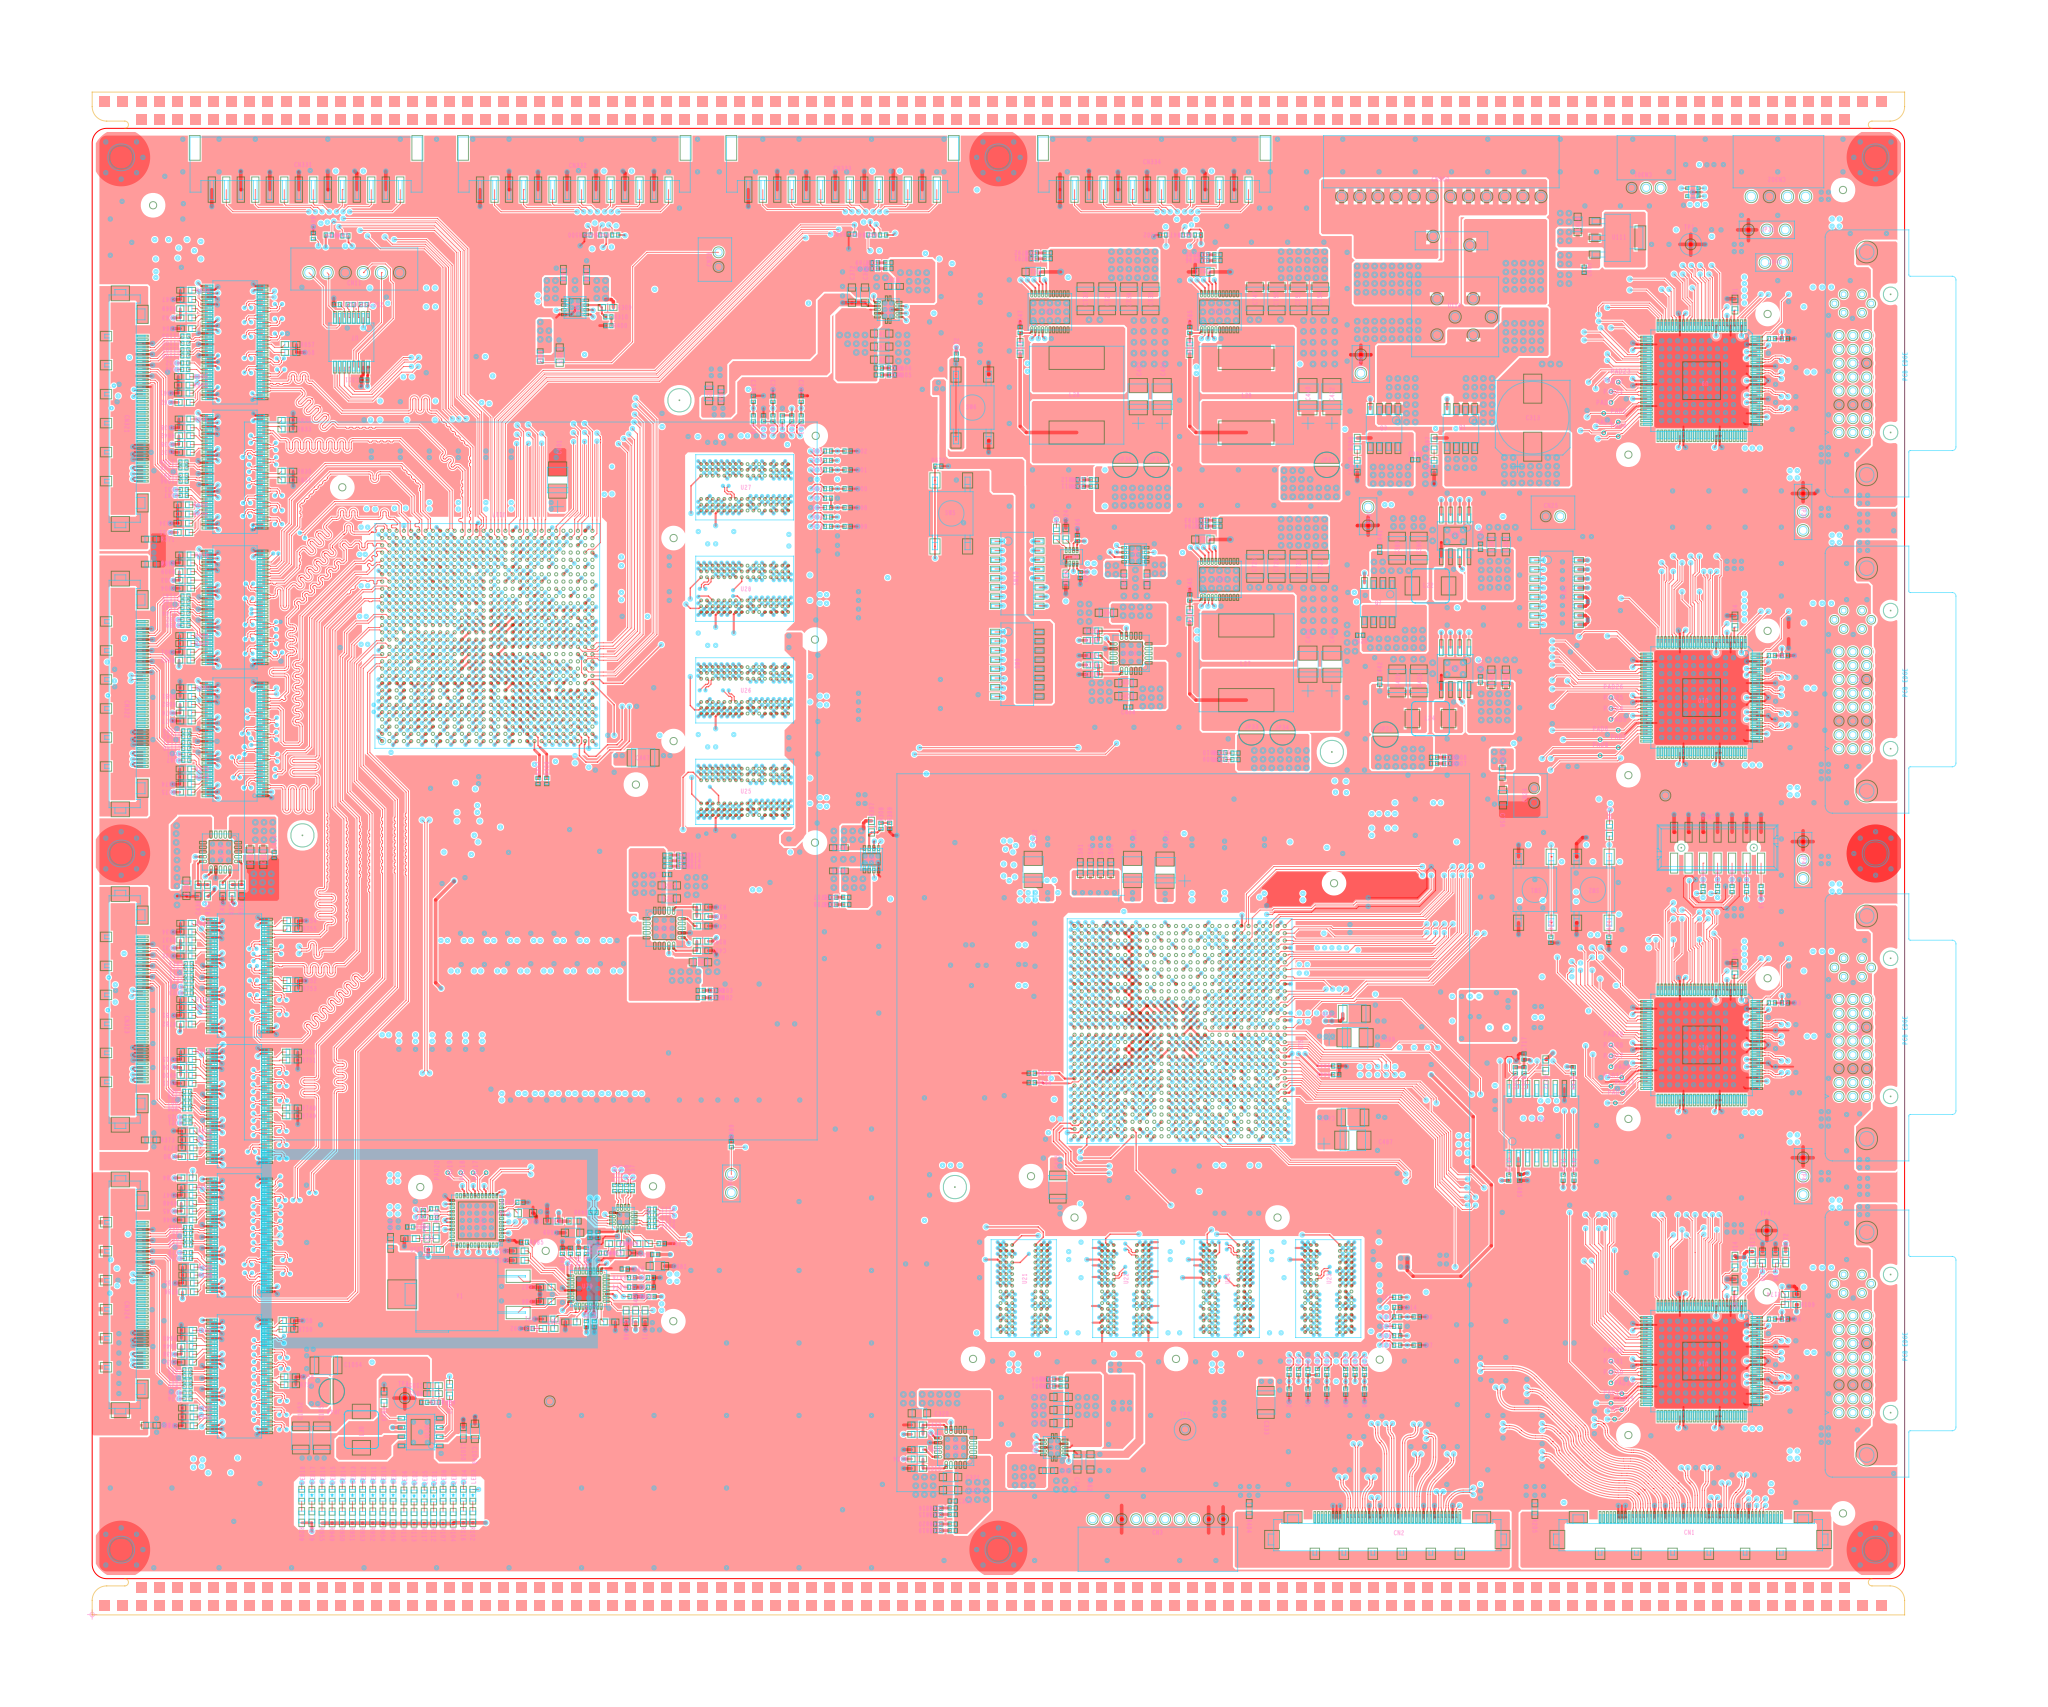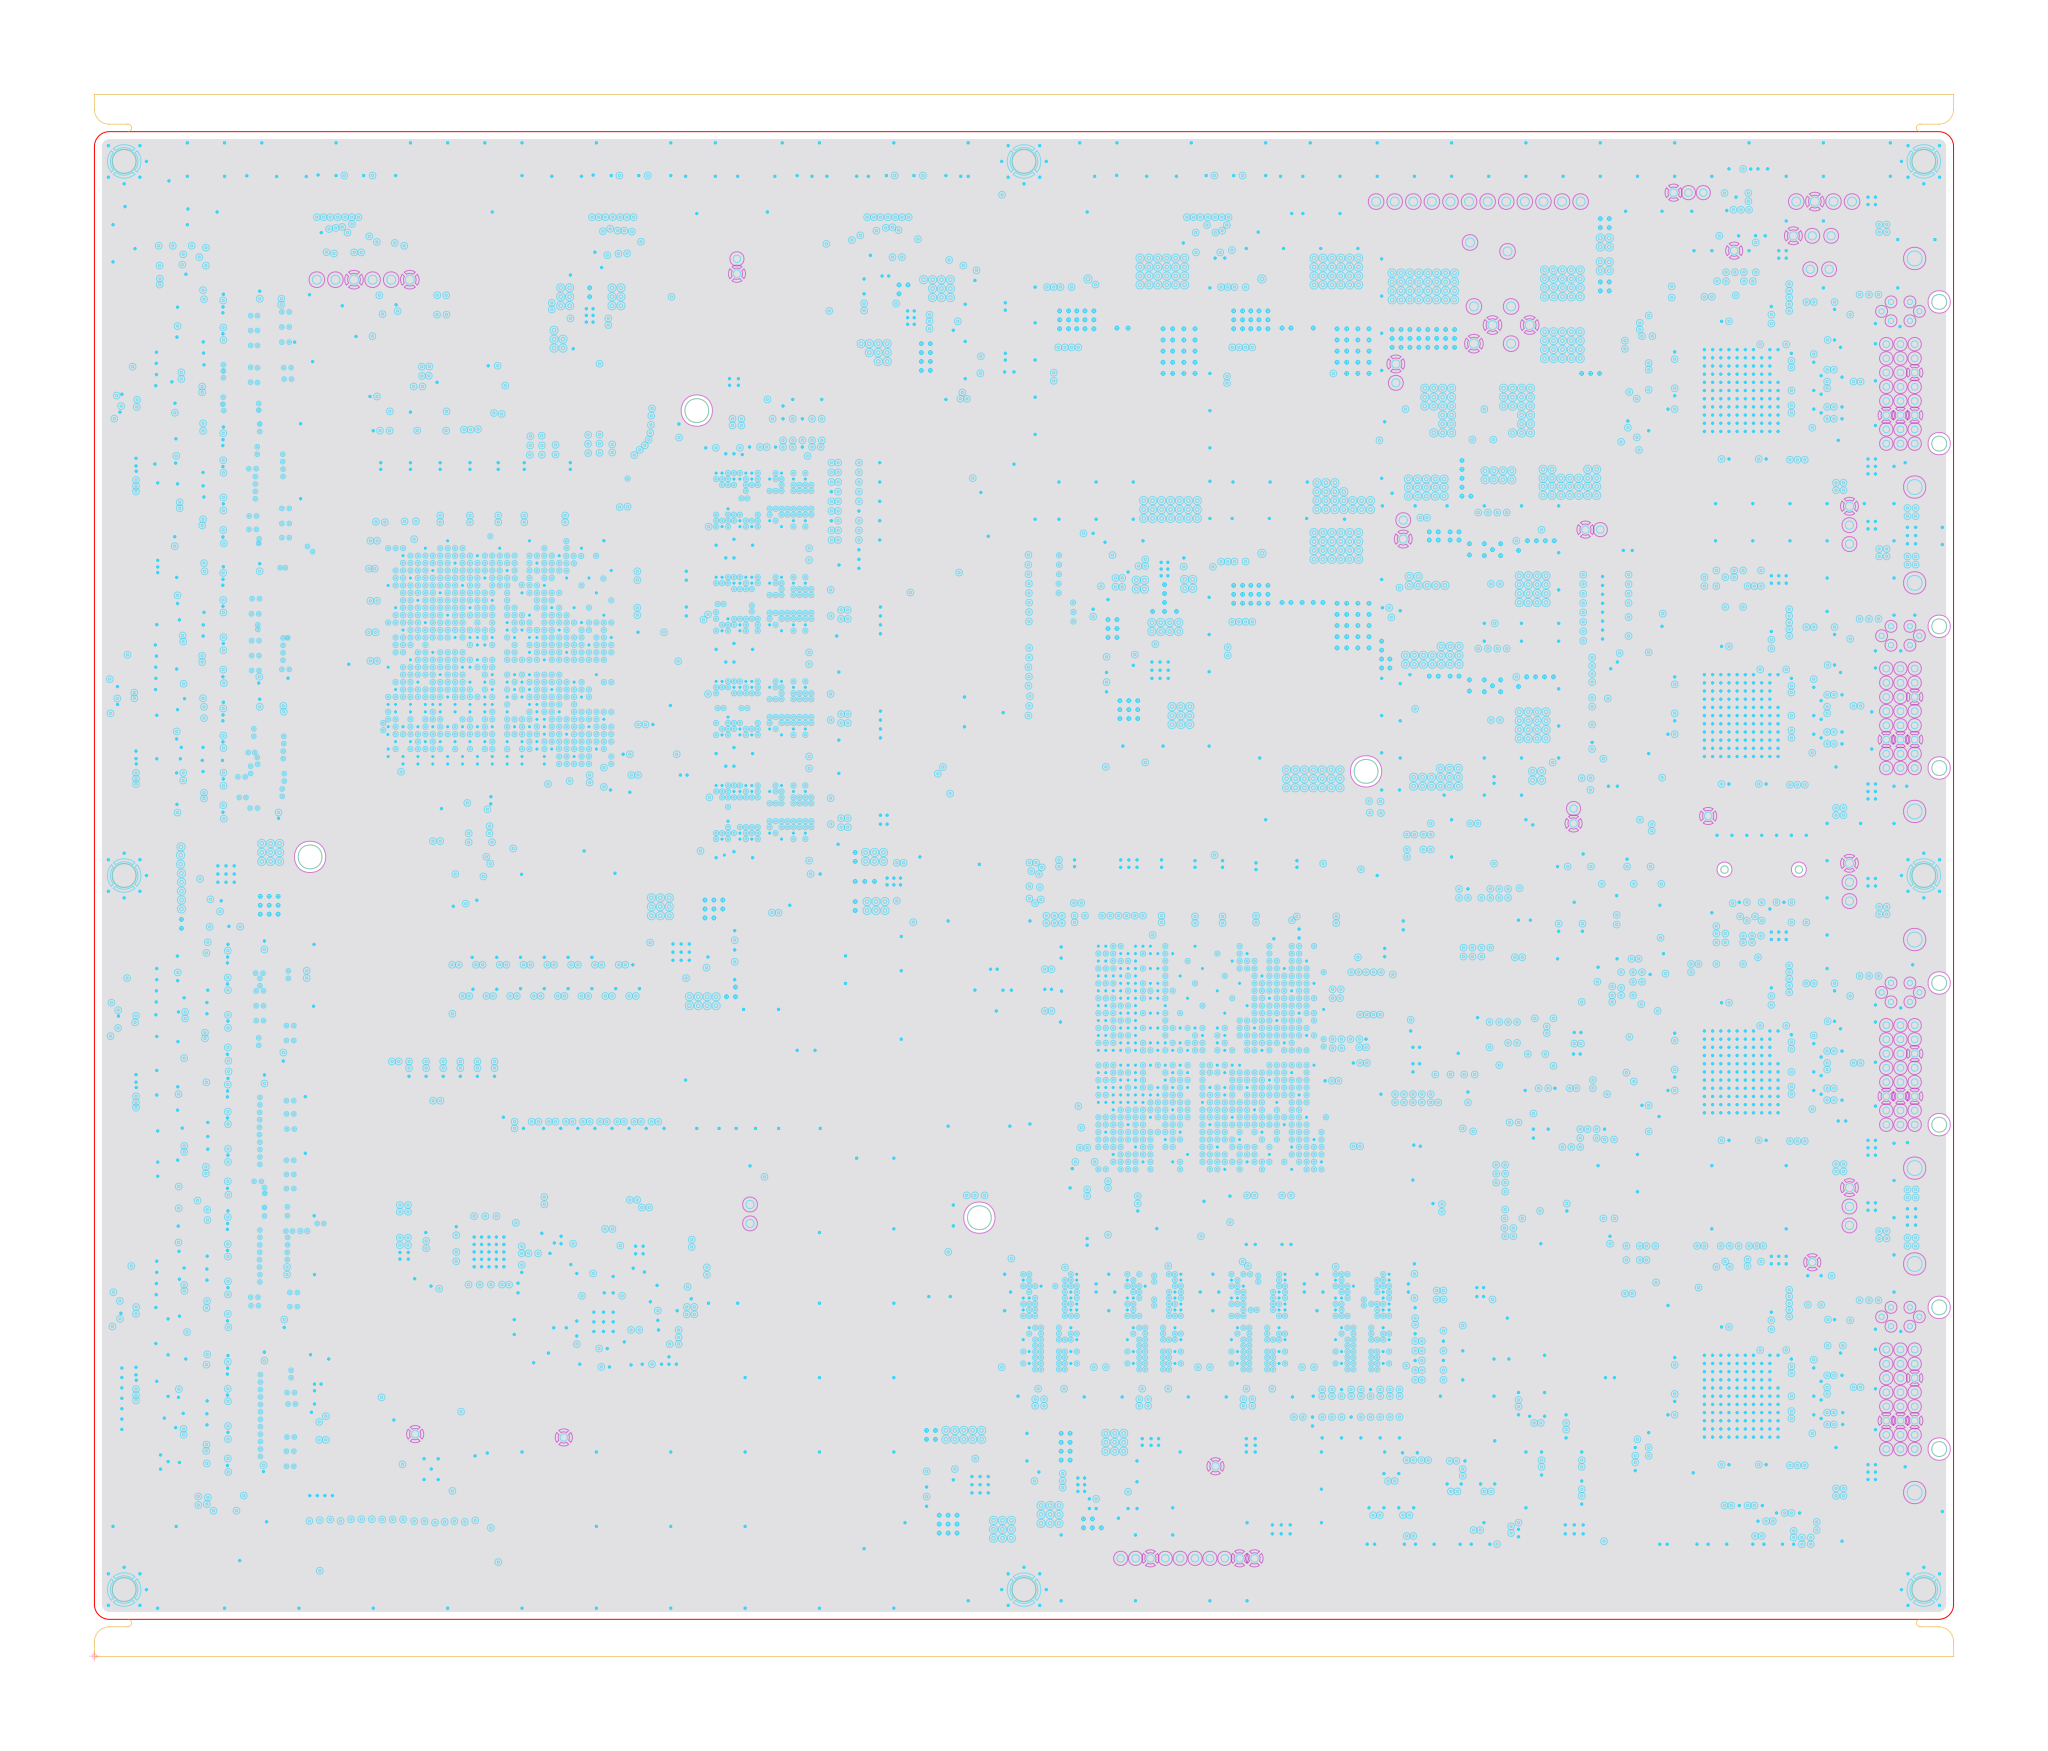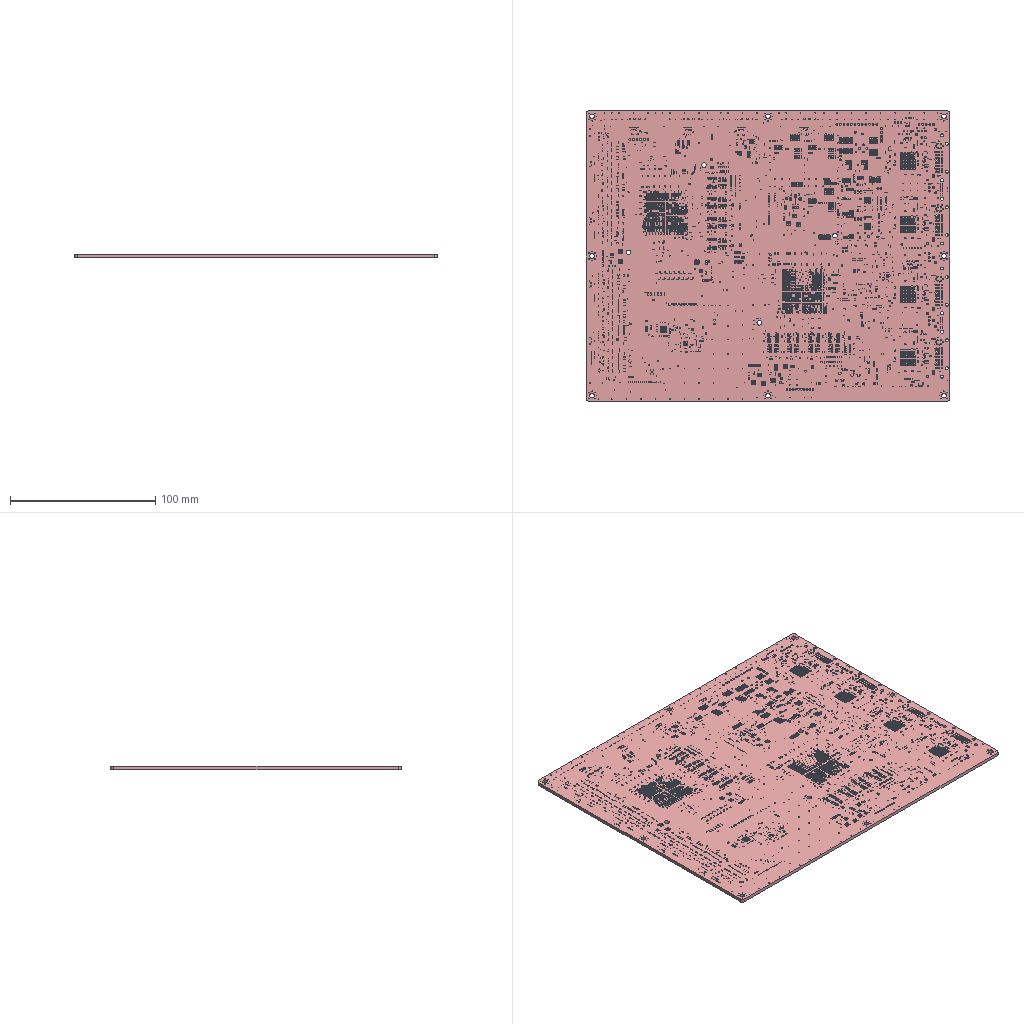Circuit board layout | Cadence Allegro | box 250 x 200 x 2.3 mm
Layer stack:
# Cadence Allegro layer stack of  (unit mm; from the constraint file cross-section; dielectric type: 0 not recorded (Allegro does not mark core vs prepreg), 3 surface material)
index,name,kind,layer,copper_thickness_mm,dielectric_type,dielectric_thickness_mm,dielectric_material,dielectric_constant
0,Top Surface,other,,,,,,
1,TOP,copper,TOP,0.0305,,,,
2,Dielectric1,dielectric,,,0,0.2032,FR-4,4.5
3,P2,copper,P2,0.0305,,,,
4,Dielectric2,dielectric,,,0,0.2032,FR-4,4.5
5,P3,copper,P3,0.0305,,,,
6,Dielectric3,dielectric,,,0,0.2032,FR-4,4.5
7,P4,copper,P4,0.0305,,,,
8,Dielectric4,dielectric,,,0,0.2032,FR-4,4.5
9,P5,copper,P5,0.0305,,,,
10,Dielectric5,dielectric,,,0,0.2032,FR-4,4.5
11,P6,copper,P6,0.0305,,,,
12,Dielectric6,dielectric,,,0,0.2032,FR-4,4.5
13,P7,copper,P7,0.0305,,,,
14,Dielectric7,dielectric,,,0,0.2032,FR-4,4.5
15,P8,copper,P8,0.0305,,,,
16,Dielectric8,dielectric,,,0,0.2032,FR-4,4.5
17,P9,copper,P9,0.0305,,,,
18,Dielectric9,dielectric,,,0,0.2032,FR-4,4.5
19,P10,copper,P10,0.0305,,,,
20,Dielectric10,dielectric,,,0,0.2032,FR-4,4.5
21,P11,copper,P11,0.0305,,,,
22,Dielectric11,dielectric,,,0,0,FR-4,1
23,BOTTOM,copper,BOTTOM,0.0305,,,,
24,Bottom Surface,other,,,,,,
# drill layer pairs: low layer,high layer
drill_pair,TOP,BOTTOM
Part placement, first 417 of 1713 lines:
REFDES,COMP_VALUE,SYM_NAME,SYM_X,SYM_Y,SYM_ROTATE,SYM_MIRROR
C1,0.1uF,CRC1005RZAS,9192.913,6927.283,0.000,NO
C2,0.1uF,CRC1005RZAS,9192.913,5206.811,0.000,NO
C3,0.1uF,CRC1005RZAS,9047.244,6576.890,180.000,YES
C4,0.1uF,CRC1005RZAS,9047.244,6624.134,180.000,YES
C5,0.1uF,CRC1005RZAS,9047.244,6698.937,180.000,YES
C6,0.1uF,CRC1005RZAS,9047.244,6805.236,180.000,YES
C7,2.2uF,CRC1608RZAS,8933.071,6443.031,0.000,YES
C8,10uF,CRC2012RZAS,8921.260,6380.039,0.000,YES
C9,0.1uF,CRC1005RZAS,9047.244,4856.417,180.000,YES
C10,0.1uF,CRC1005RZAS,9047.244,4903.661,180.000,YES
C11,0.1uF,CRC1005RZAS,9047.244,4978.465,180.000,YES
C12,0.1uF,CRC1005RZAS,9047.244,5084.764,180.000,YES
C13,2.2uF,CRC1608RZAS,8933.071,4722.559,0.000,YES
C14,10uF,CRC2012RZAS,8921.260,4659.567,0.000,YES
C15,0.1uF,CRC1005RZAS,8811.024,6380.039,180.000,YES
C16,0.1uF,CRC1005RZAS,8401.575,6691.063,90.000,YES
C17,0.1uF,CRC1005RZAS,8877.953,6994.213,90.000,YES
C18,2.2uF,CRC1608RZAS,8858.268,7289.488,270.000,YES
C19,10uF,CRC2012RZAS,8925.197,7301.299,270.000,YES
C20,0.1uF,CRC1005RZAS,8811.024,4659.567,180.000,YES
C21,0.1uF,CRC1005RZAS,8401.575,4970.591,90.000,YES
C22,0.1uF,CRC1005RZAS,8877.953,5273.740,90.000,YES
C23,2.2uF,CRC1608RZAS,8858.268,5569.016,270.000,YES
C24,10uF,CRC2012RZAS,8925.197,5580.827,270.000,YES
C25,0.1uF,CRC1005RZAS,9145.669,6502.087,180.000,YES
C26,0.1uF,CRC1005RZAS,8633.858,6372.165,180.000,YES
C27,0.1uF,CRC1005RZAS,8633.858,7029.646,0.000,YES
C28,0.1uF,CRC1005RZAS,8401.575,6883.976,270.000,YES
C29,2.2uF,CRC1608RZAS,9287.402,6324.921,180.000,YES
C30,10uF,CRC2012RZAS,9295.276,6257.992,180.000,YES
C31,0.1uF,CRC1005RZAS,8633.858,4651.693,180.000,YES
C32,0.1uF,CRC1005RZAS,9145.669,4781.614,180.000,YES
C33,0.1uF,CRC1005RZAS,8401.575,5163.504,270.000,YES
C34,0.1uF,CRC1005RZAS,8633.858,5309.173,0.000,YES
C35,2.2uF,CRC1608RZAS,9287.402,4604.449,180.000,YES
C36,10uF,CRC2012RZAS,9295.276,4537.520,180.000,YES
C37,0.1uF,CRC1005RZAS,9047.244,6891.850,0.000,YES
C38,2.2uF,CRC1608RZAS,9051.181,6946.969,0.000,YES
C39,10uF,CRC2012RZAS,9055.118,7069.016,180.000,YES
C40,0.1uF,CRC1005RZAS,9047.244,5171.378,0.000,YES
C41,2.2uF,CRC1608RZAS,9047.244,5226.496,0.000,YES
C42,10uF,CRC2012RZAS,9055.118,5352.480,180.000,YES
C43,0.1uF,CRC1005RZAS,9192.913,3320.984,0.000,NO
C44,0.1uF,CRC1005RZAS,9192.913,1604.449,0.000,NO
C45,0.1uF,CRC1005RZAS,9047.244,3198.937,180.000,YES
C46,0.1uF,CRC1005RZAS,9047.244,2970.591,180.000,YES
C47,0.1uF,CRC1005RZAS,9047.244,3017.835,180.000,YES
C48,0.1uF,CRC1005RZAS,9047.244,3092.638,180.000,YES
C49,2.2uF,CRC1608RZAS,8933.071,2836.732,0.000,YES
C50,10uF,CRC2012RZAS,8921.260,2773.740,0.000,YES
C51,0.1uF,CRC1005RZAS,9047.244,1254.055,180.000,YES
C52,0.1uF,CRC1005RZAS,9047.244,1301.299,180.000,YES
C53,0.1uF,CRC1005RZAS,9047.244,1376.102,180.000,YES
C54,0.1uF,CRC1005RZAS,9047.244,1482.402,180.000,YES
C55,2.2uF,CRC1608RZAS,8933.071,1120.197,0.000,YES
C56,10uF,CRC2012RZAS,8925.197,1053.268,0.000,YES
C57,0.1uF,CRC1005RZAS,8811.024,2773.740,180.000,YES
C58,0.1uF,CRC1005RZAS,8401.575,3084.764,90.000,YES
C59,0.1uF,CRC1005RZAS,8877.953,3387.913,90.000,YES
C60,2.2uF,CRC1608RZAS,8858.268,3683.189,270.000,YES
C61,10uF,CRC2012RZAS,8925.197,3695.000,270.000,YES
C62,0.1uF,CRC1005RZAS,8811.024,1057.205,180.000,YES
C63,0.1uF,CRC1005RZAS,8877.953,1671.378,90.000,YES
C64,0.1uF,CRC1005RZAS,8401.575,1368.228,90.000,YES
C65,2.2uF,CRC1608RZAS,8858.268,1966.654,270.000,YES
C66,10uF,CRC2012RZAS,8925.197,1978.465,270.000,YES
C67,0.1uF,CRC1005RZAS,8401.575,3277.677,270.000,YES
C68,0.1uF,CRC1005RZAS,8633.858,2765.866,180.000,YES
C69,0.1uF,CRC1005RZAS,9145.669,2895.787,180.000,YES
C70,0.1uF,CRC1005RZAS,8633.858,3423.346,0.000,YES
C71,2.2uF,CRC1608RZAS,9287.402,2718.622,180.000,YES
C72,10uF,CRC2012RZAS,9295.276,2651.693,180.000,YES
C73,0.1uF,CRC1005RZAS,8633.858,1049.331,180.000,YES
C74,0.1uF,CRC1005RZAS,9145.669,1179.252,180.000,YES
C75,0.1uF,CRC1005RZAS,8401.575,1561.142,270.000,YES
C76,0.1uF,CRC1005RZAS,8633.858,1706.811,0.000,YES
C77,2.2uF,CRC1608RZAS,9287.402,1002.087,180.000,YES
C78,10uF,CRC2012RZAS,9295.276,935.157,180.000,YES
C79,0.1uF,CRC1005RZAS,9047.244,3285.551,0.000,YES
C80,2.2uF,CRC1608RZAS,9047.244,3340.669,0.000,YES
C81,10uF,CRC2012RZAS,9055.118,3462.717,180.000,YES
C82,0.1uF,CRC1005RZAS,9047.244,1569.016,0.000,YES
C83,2.2uF,CRC1608RZAS,9047.244,1624.134,0.000,YES
C84,10uF,CRC2012RZAS,9055.118,1746.181,180.000,YES
C85,0.1uF,CRC1005RZAS,7192.913,1750.118,0.000,YES
C86,0.1uF,CRC1005RZAS,7192.913,1616.260,0.000,NO
C87,0.1uF,CRC1005RZAS,7192.913,1462.717,0.000,NO
C88,0.1uF,CRC1005RZAS,6909.449,1210.748,270.000,NO
C89,0.1uF,CRC1005RZAS,6807.087,1210.748,270.000,NO
C90,0.1uF,CRC1005RZAS,6704.724,1210.748,270.000,NO
C91,0.1uF,CRC1005RZAS,6602.362,1210.748,270.000,NO
C92,0.1uF,CRC1005RZAS,6500.000,1210.748,270.000,NO
C93,0.1uF,CRC1005RZAS,5240.157,1817.047,270.000,YES
C94,0.1uF,CRC1005RZAS,5251.969,1883.976,180.000,YES
C95,0.1uF,CRC1005RZAS,5251.969,1970.591,180.000,YES
C96,0.1uF,CRC1005RZAS,5188.976,2061.142,180.000,YES
C97,2.2uF,CRC1608RZAS,4980.315,1250.118,90.000,YES
C98,10uF,CRC2012RZAS,5047.244,1238.307,90.000,YES
C99,0.1uF,CRC1005RZAS,4901.575,1927.283,0.000,YES
C100,0.1uF,CRC1005RZAS,4948.819,1769.803,0.000,YES
C101,0.1uF,CRC1005RZAS,4870.079,2021.772,0.000,YES
C102,0.1uF,CRC1005RZAS,4870.079,1970.591,0.000,YES
C103,0.1uF,CRC1005RZAS,4881.890,1868.228,270.000,YES
C104,10uF,CRC2012RZAS,5220.472,1415.472,180.000,YES
C105,2.2uF,CRC1608RZAS,4921.260,1415.472,0.000,YES
C106,0.1uF,CRC1005RZAS,4933.071,1580.827,180.000,YES
C107,0.1uF,CRC1005RZAS,4933.071,1643.819,180.000,YES
C108,2200pF,CRC1608RZAS,5291.339,1683.189,270.000,YES
C109,0.22uF,CRC1608RZAS,5240.157,1683.189,270.000,YES
C110,0.1uF,CRC1005RZAS,5019.685,1769.803,180.000,YES
C111,0.1uF,CRC1005RZAS,5185.039,1517.835,0.000,YES
C112,0.1uF,CRC1005RZAS,5185.039,1580.827,0.000,YES
C113,0.1uF,CRC1005RZAS,5137.795,1722.559,270.000,YES
C114,0.1uF,CRC1005RZAS,5090.551,1832.795,0.000,YES
C115,0.1uF,CRC1005RZAS,5251.969,1927.283,180.000,YES
C116,0.1uF,CRC1005RZAS,4996.063,1990.276,180.000,YES
C117,2200pF,CRC1608RZAS,4850.394,1714.685,0.000,YES
C118,0.22uF,CRC1608RZAS,4850.394,1765.866,0.000,YES
C119,10uF,CRC2012RZAS,5771.654,1415.472,180.000,YES
C120,2.2uF,CRC1608RZAS,5472.441,1415.472,0.000,YES
C121,0.1uF,CRC1005RZAS,5736.220,1517.835,0.000,YES
C122,0.1uF,CRC1005RZAS,5736.220,1580.827,0.000,YES
C123,0.1uF,CRC1005RZAS,5688.976,1722.559,270.000,YES
C124,0.1uF,CRC1005RZAS,5484.252,1580.827,180.000,YES
C125,0.1uF,CRC1005RZAS,5484.252,1643.819,180.000,YES
C126,0.1uF,CRC1005RZAS,5570.866,1769.803,180.000,YES
C127,0.1uF,CRC1005RZAS,5641.732,1820.984,0.000,YES
C128,0.1uF,CRC1005RZAS,5803.150,1927.283,180.000,YES
C129,0.1uF,CRC1005RZAS,5547.244,1990.276,180.000,YES
C130,0.1uF,CRC1005RZAS,5791.339,1817.047,270.000,YES
C131,0.1uF,CRC1005RZAS,5803.150,1883.976,180.000,YES
C132,0.1uF,CRC1005RZAS,5803.150,1970.591,180.000,YES
C133,0.1uF,CRC1005RZAS,5736.220,2061.142,180.000,YES
C134,2.2uF,CRC1608RZAS,5531.496,1250.118,90.000,YES
C135,10uF,CRC2012RZAS,5598.425,1238.307,90.000,YES
C136,0.1uF,CRC1005RZAS,5421.260,2021.772,0.000,YES
C137,0.1uF,CRC1005RZAS,5421.260,1970.591,0.000,YES
C138,0.1uF,CRC1005RZAS,5452.756,1927.283,0.000,YES
C139,0.1uF,CRC1005RZAS,5433.071,1868.228,270.000,YES
C140,0.1uF,CRC1005RZAS,5500.000,1769.803,0.000,YES
C141,2200pF,CRC1608RZAS,5842.520,1683.189,270.000,YES
C142,0.22uF,CRC1608RZAS,5791.339,1683.189,270.000,YES
C143,2200pF,CRC1608RZAS,5401.575,1714.685,0.000,YES
C144,0.22uF,CRC1608RZAS,5401.575,1765.866,0.000,YES
C145,10uF,CRC2012RZAS,7035.433,2065.079,270.000,YES
C146,2.2uF,CRC1608RZAS,7035.433,1876.102,90.000,YES
C147,0.1uF,CRC1005RZAS,6586.614,1580.827,180.000,YES
C148,0.1uF,CRC1005RZAS,6586.614,1643.819,180.000,YES
C149,0.1uF,CRC1005RZAS,6838.583,1517.835,0.000,YES
C150,0.1uF,CRC1005RZAS,6838.583,1580.827,0.000,YES
C151,0.1uF,CRC1005RZAS,6791.339,1722.559,270.000,YES
C152,0.1uF,CRC1005RZAS,6673.228,1769.803,180.000,YES
C153,0.1uF,CRC1005RZAS,6905.512,1927.283,180.000,YES
C154,0.1uF,CRC1005RZAS,6649.606,1990.276,180.000,YES
C155,0.1uF,CRC1005RZAS,6744.094,1820.984,0.000,YES
C156,0.1uF,CRC1005RZAS,6893.701,1817.047,270.000,YES
C157,0.1uF,CRC1005RZAS,6905.512,1883.976,180.000,YES
C158,0.1uF,CRC1005RZAS,6905.512,1970.591,180.000,YES
C159,0.1uF,CRC1005RZAS,6838.583,2061.142,180.000,YES
C160,2.2uF,CRC1608RZAS,7216.535,1887.913,180.000,YES
C161,10uF,CRC2012RZAS,7228.346,1954.843,180.000,YES
C162,0.1uF,CRC1005RZAS,6602.362,1769.803,0.000,YES
C163,0.1uF,CRC1005RZAS,6535.433,1868.228,270.000,YES
C164,0.1uF,CRC1005RZAS,6555.118,1927.283,0.000,YES
C165,0.1uF,CRC1005RZAS,6523.622,1970.591,0.000,YES
C166,0.1uF,CRC1005RZAS,6523.622,2021.772,0.000,YES
C167,2200pF,CRC1608RZAS,6944.882,1687.126,270.000,YES
C168,0.22uF,CRC1608RZAS,6893.701,1687.126,270.000,YES
C169,2200pF,CRC1608RZAS,6503.937,1714.685,0.000,YES
C170,0.22uF,CRC1608RZAS,6503.937,1765.866,0.000,YES
C171,10uF,CRC2012RZAS,6322.835,1415.472,180.000,YES
C172,2.2uF,CRC1608RZAS,6023.622,1415.472,0.000,YES
C173,0.1uF,CRC1005RZAS,6287.402,1517.835,0.000,YES
C174,0.1uF,CRC1005RZAS,6287.402,1580.827,0.000,YES
C175,0.1uF,CRC1005RZAS,6240.157,1722.559,270.000,YES
C176,0.1uF,CRC1005RZAS,6192.913,1805.236,0.000,YES
C177,0.1uF,CRC1005RZAS,6354.331,1927.283,180.000,YES
C178,0.1uF,CRC1005RZAS,6035.433,1580.827,180.000,YES
C179,0.1uF,CRC1005RZAS,6035.433,1643.819,180.000,YES
C180,0.1uF,CRC1005RZAS,6122.047,1769.803,180.000,YES
C181,0.1uF,CRC1005RZAS,6098.425,1990.276,180.000,YES
C182,0.1uF,CRC1005RZAS,5984.252,1868.228,270.000,YES
C183,0.1uF,CRC1005RZAS,6003.937,1927.283,0.000,YES
C184,0.1uF,CRC1005RZAS,5972.441,1970.591,0.000,YES
C185,0.1uF,CRC1005RZAS,5972.441,2021.772,0.000,YES
C186,2.2uF,CRC1608RZAS,6082.677,1250.118,90.000,YES
C187,10uF,CRC2012RZAS,6149.606,1238.307,90.000,YES
C188,0.1uF,CRC1005RZAS,6342.520,1817.047,270.000,YES
C189,0.1uF,CRC1005RZAS,6354.331,1883.976,180.000,YES
C190,0.1uF,CRC1005RZAS,6354.331,1970.591,180.000,YES
C191,0.1uF,CRC1005RZAS,6287.402,2061.142,180.000,YES
C192,0.1uF,CRC1005RZAS,6051.181,1769.803,0.000,YES
C193,2200pF,CRC1608RZAS,6393.701,1683.189,270.000,YES
C194,0.22uF,CRC1608RZAS,6342.520,1683.189,270.000,YES
C195,2200pF,CRC1608RZAS,5952.756,1765.866,0.000,YES
C196,0.22uF,CRC1608RZAS,5952.756,1714.685,0.000,YES
C197,0.1uF,CRC1005RZAS,3562.992,6600.512,90.000,YES
C198,0.1uF,CRC1005RZAS,4102.362,6009.961,0.000,NO
C199,0.1uF,CRC1005RZAS,4102.362,5907.598,0.000,NO
C200,0.1uF,CRC1005RZAS,4102.362,6112.323,0.000,NO
C201,0.1uF,CRC1005RZAS,4102.362,6214.685,0.000,NO
C202,0.1uF,CRC1005RZAS,4102.362,6317.047,0.000,NO
C203,0.1uF,CRC1005RZAS,3696.850,6600.512,90.000,NO
C204,0.1uF,CRC1005RZAS,3850.394,6600.512,90.000,NO
C205,0.1uF,CRC1005RZAS,3251.969,4596.575,270.000,YES
C206,0.1uF,CRC1005RZAS,3342.520,4659.567,270.000,YES
C207,0.1uF,CRC1005RZAS,3429.134,4659.567,270.000,YES
C208,0.1uF,CRC1005RZAS,3496.063,4647.756,0.000,YES
C209,2.2uF,CRC1608RZAS,3415.000,6620.000,90.000,NO
C210,10uF,CRC2012RZAS,3350.000,6630.000,90.000,NO
C211,0.1uF,CRC1005RZAS,3543.307,4356.417,90.000,YES
C212,0.1uF,CRC1005RZAS,3444.882,4289.488,0.000,YES
C213,0.1uF,CRC1005RZAS,3385.827,4309.173,90.000,YES
C214,0.1uF,CRC1005RZAS,3342.520,4277.677,90.000,YES
C215,0.1uF,CRC1005RZAS,3291.339,4277.677,90.000,YES
C216,10uF,CRC2012RZAS,3248.031,6443.031,0.000,YES
C217,2.2uF,CRC1608RZAS,3437.008,6443.031,180.000,YES
C218,0.1uF,CRC1005RZAS,3590.551,4545.394,0.000,YES
C219,0.1uF,CRC1005RZAS,3480.315,4498.150,90.000,YES
C220,0.1uF,CRC1005RZAS,3322.835,4403.661,270.000,YES
C221,0.1uF,CRC1005RZAS,3385.827,4659.567,270.000,YES
C222,0.1uF,CRC1005RZAS,3732.283,4592.638,90.000,YES
C223,0.1uF,CRC1005RZAS,3795.276,4592.638,90.000,YES
C224,0.1uF,CRC1005RZAS,3732.283,4340.669,270.000,YES
C225,0.1uF,CRC1005RZAS,3669.291,4340.669,270.000,YES
C226,2200pF,CRC1608RZAS,3629.921,4698.937,0.000,YES
C227,0.22uF,CRC1608RZAS,3629.921,4647.756,0.000,YES
C228,2200pF,CRC1608RZAS,3547.244,4257.992,90.000,YES
C229,0.22uF,CRC1608RZAS,3598.425,4257.992,90.000,YES
C230,0.1uF,CRC1005RZAS,3543.307,4427.283,270.000,YES
C231,10uF,CRC2012RZAS,3897.638,5179.252,270.000,YES
C232,2.2uF,CRC1608RZAS,3897.638,4880.039,90.000,YES
C233,0.1uF,CRC1005RZAS,3385.827,5210.748,270.000,YES
C234,0.1uF,CRC1005RZAS,3732.283,5143.819,90.000,YES
C235,0.1uF,CRC1005RZAS,3795.276,5143.819,90.000,YES
C236,0.1uF,CRC1005RZAS,3322.835,4954.843,270.000,YES
C237,0.1uF,CRC1005RZAS,3492.126,5049.331,90.000,YES
C238,0.1uF,CRC1005RZAS,3590.551,5096.575,0.000,YES
C239,0.1uF,CRC1005RZAS,3543.307,4978.465,270.000,YES
C240,0.1uF,CRC1005RZAS,3669.291,4891.850,270.000,YES
C241,0.1uF,CRC1005RZAS,3732.283,4891.850,270.000,YES
C242,0.1uF,CRC1005RZAS,3251.969,5143.819,270.000,YES
C243,0.1uF,CRC1005RZAS,3342.520,5210.748,270.000,YES
C244,0.1uF,CRC1005RZAS,3429.134,5210.748,270.000,YES
C245,0.1uF,CRC1005RZAS,3496.063,5198.937,0.000,YES
C246,2.2uF,CRC1608RZAS,4062.992,4939.094,180.000,YES
C247,10uF,CRC2012RZAS,4074.803,5006.024,180.000,YES
C248,0.1uF,CRC1005RZAS,3543.307,4907.598,90.000,YES
C249,0.1uF,CRC1005RZAS,3444.882,4840.669,0.000,YES
C250,0.1uF,CRC1005RZAS,3385.827,4860.354,90.000,YES
C251,0.1uF,CRC1005RZAS,3342.520,4828.858,90.000,YES
C252,0.1uF,CRC1005RZAS,3291.339,4828.858,90.000,YES
C253,2200pF,CRC1608RZAS,3629.921,5250.118,0.000,YES
C254,0.22uF,CRC1608RZAS,3629.921,5198.937,0.000,YES
C255,2200pF,CRC1608RZAS,3547.244,4809.173,90.000,YES
C256,0.22uF,CRC1608RZAS,3598.425,4809.173,90.000,YES
C257,10uF,CRC2012RZAS,3897.638,4628.071,270.000,YES
C258,2.2uF,CRC1608RZAS,3897.638,4328.858,90.000,YES
C259,0.1uF,CRC1005RZAS,3543.307,6080.827,270.000,YES
C260,0.1uF,CRC1005RZAS,3385.827,6313.110,270.000,YES
C261,0.1uF,CRC1005RZAS,3732.283,6246.181,90.000,YES
C262,0.1uF,CRC1005RZAS,3795.276,6246.181,90.000,YES
C263,0.1uF,CRC1005RZAS,3322.835,6057.205,270.000,YES
C264,0.1uF,CRC1005RZAS,3492.126,6151.693,90.000,YES
C265,0.1uF,CRC1005RZAS,3669.291,5994.213,270.000,YES
C266,0.1uF,CRC1005RZAS,3732.283,5994.213,270.000,YES
C267,0.1uF,CRC1005RZAS,3590.551,6198.937,0.000,YES
C268,0.1uF,CRC1005RZAS,3251.969,6246.181,270.000,YES
C269,0.1uF,CRC1005RZAS,3342.520,6313.110,270.000,YES
C270,0.1uF,CRC1005RZAS,3429.134,6313.110,270.000,YES
C271,0.1uF,CRC1005RZAS,3496.063,6301.299,0.000,YES
C272,2.2uF,CRC1608RZAS,4062.992,4387.913,180.000,YES
C273,10uF,CRC2012RZAS,4074.803,4454.843,180.000,YES
C274,0.1uF,CRC1005RZAS,3291.339,5931.220,90.000,YES
C275,0.1uF,CRC1005RZAS,3385.827,5962.717,90.000,YES
C276,0.1uF,CRC1005RZAS,3444.882,5943.031,0.000,YES
C277,0.1uF,CRC1005RZAS,3342.520,5931.220,90.000,YES
C278,0.1uF,CRC1005RZAS,3543.307,6009.961,90.000,YES
C279,2200pF,CRC1608RZAS,3625.984,6352.480,0.000,YES
C280,0.22uF,CRC1608RZAS,3625.984,6301.299,0.000,YES
C281,2200pF,CRC1608RZAS,3598.425,5911.535,90.000,YES
C282,0.22uF,CRC1608RZAS,3547.244,5911.535,90.000,YES
C283,10uF,CRC2012RZAS,3897.638,5730.433,270.000,YES
C284,2.2uF,CRC1608RZAS,3897.638,5431.220,90.000,YES
C285,0.1uF,CRC1005RZAS,3669.291,5443.031,270.000,YES
C286,0.1uF,CRC1005RZAS,3543.307,5529.646,270.000,YES
C287,0.1uF,CRC1005RZAS,3322.835,5506.024,270.000,YES
C288,0.1uF,CRC1005RZAS,3385.827,5761.929,270.000,YES
C289,0.1uF,CRC1005RZAS,3732.283,5695.000,90.000,YES
C290,0.1uF,CRC1005RZAS,3795.276,5695.000,90.000,YES
C291,0.1uF,CRC1005RZAS,3732.283,5443.031,270.000,YES
C292,0.1uF,CRC1005RZAS,3507.874,5600.512,90.000,YES
C293,0.1uF,CRC1005RZAS,3590.551,5647.756,0.000,YES
C294,0.1uF,CRC1005RZAS,3342.520,5761.929,270.000,YES
C295,0.1uF,CRC1005RZAS,3429.134,5761.929,270.000,YES
C296,0.1uF,CRC1005RZAS,3496.063,5750.118,0.000,YES
C297,0.1uF,CRC1005RZAS,3291.339,5380.039,90.000,YES
C298,2.2uF,CRC1608RZAS,4062.992,5490.276,180.000,YES
C299,10uF,CRC2012RZAS,4074.803,5557.205,180.000,YES
C300,0.1uF,CRC1005RZAS,3251.969,5695.000,270.000,YES
C301,0.1uF,CRC1005RZAS,3342.520,5380.039,90.000,YES
C302,0.1uF,CRC1005RZAS,3385.827,5411.535,90.000,YES
C303,0.1uF,CRC1005RZAS,3444.882,5391.850,0.000,YES
C304,0.1uF,CRC1005RZAS,3543.307,5458.780,90.000,YES
C305,2200pF,CRC1608RZAS,3629.921,5801.299,0.000,YES
C306,0.22uF,CRC1608RZAS,3629.921,5750.118,0.000,YES
C307,2200pF,CRC1608RZAS,3598.425,5360.354,90.000,YES
C308,0.22uF,CRC1608RZAS,3547.244,5360.354,90.000,YES
C309,0.1uF,CRC1005RZAS,7401.575,6620.197,90.000,YES
C310,0.1uF,CRC1005RZAS,1328.976,7112.323,0.000,NO
C311,0.1uF,CRC1005RZAS,1478.583,6702.874,180.000,NO
C312,0.1uF,CRC1005RZAS,1474.646,7112.323,0.000,NO
C313,470uF/25V,CEC100RZAS,7822.835,6498.150,90.000,NO
C314,0.1uF,CRC1005RZAS,1425.000,6984.999,180.000,YES
C315,0.1uF,CRC1005RZAS,1403.780,7112.323,0.000,NO
C316,0.1uF,CRC1005RZAS,9295.276,7151.693,270.000,YES
C317,0.1uF,CRC1005RZAS,9295.276,5435.157,270.000,YES
C318,0.1uF,CRC1005RZAS,9295.276,3545.394,270.000,YES
C319,0.1uF,CRC1005RZAS,7905.512,6336.732,270.000,YES
C320,10uF,CRC2012RZAS,4492.126,1092.638,0.000,NO
C321,10uF,CRC2012RZAS,4661.417,746.181,0.000,NO
C322,10uF,CRC2012RZAS,3303.150,3541.457,180.000,NO
C323,10uF,CRC2012RZAS,3133.858,3887.913,180.000,NO
C324,100pF_NMT,CRC1608RZAS,5287.402,5868.228,270.000,NO
C325,0.1uF,CRC1005RZAS,4673.228,616.260,0.000,NO
C326,10uF,CRC2012RZAS,4661.417,675.315,0.000,NO
C327,0.1uF,CRC1005RZAS,3122.047,4017.835,180.000,NO
C328,10uF,CRC2012RZAS,3133.858,3958.780,180.000,NO
C329,0.1uF,CRC1005RZAS,7921.260,3663.504,90.000,NO
C330,0.1uF,CRC1005RZAS,7838.583,3860.354,270.000,YES
C331,0.1uF,CRC1005RZAS,7791.339,3860.354,270.000,YES
C332,1uF_NMT,CRC1608RZAS,7929.134,3943.031,90.000,YES
C333,22uF,CRC3225RZAS,6374.016,1151.693,270.000,NO
C334,0.1uF,CRC1005RZAS,3590.551,6600.512,90.000,NO
C335,0.1uF,CRC1005RZAS,9295.276,1828.858,270.000,YES
C337,100pF,CRC1608RZAS,2309.449,2293.425,0.000,YES
C338,0.1uF,CRC1005RZAS,2325.197,2238.307,180.000,NO
C339,100pF,CRC1608RZAS,2309.449,2344.606,0.000,YES
C340,100pF,CRC1608RZAS,2159.843,2372.165,0.000,YES
C341,100pF,CRC1608RZAS,1994.488,2285.551,180.000,YES
C342,100pF,CRC1608RZAS,2214.961,2128.071,270.000,YES
C343,100pF,CRC1608RZAS,2340.945,2069.016,0.000,YES
C344,10uF,CRC2012RZAS,2352.756,2179.252,180.000,NO
C345,10uF,CRC2012RZAS,2356.693,2187.126,0.000,YES
C346,100pF,CRC1608RZAS,2022.047,1887.913,270.000,YES
C347,100pF,CRC1608RZAS,1966.929,1887.913,270.000,YES
C348,100pF,CRC1608RZAS,1833.071,2080.827,180.000,YES
C349,10uF,CRC2012RZAS,2195.276,1880.039,270.000,YES
C350,1uF,CRC1608RZAS,1856.693,1982.402,180.000,NO
C351,100pF,CRC1608RZAS,1833.071,2238.307,180.000,YES
C352,10uF,CRC2012RZAS,5261.811,1039.488,180.000,NO
C353,10uF,CRC2012RZAS,5261.811,1110.354,180.000,NO
C354,10uF,CRC2012RZAS,5261.811,1181.220,180.000,NO
C355,100pF,CRC1608RZAS,1726.772,2041.457,0.000,NO
C356,100pF,CRC1608RZAS,1833.071,2139.882,180.000,YES
C357,100pF,CRC1608RZAS,2340.945,2013.898,0.000,YES
C358,5.6nF,CRC1608RZAS,1817.323,2072.953,270.000,NO
C359,10uF,CRC2012RZAS,1825.197,2013.898,180.000,YES
C360,1000pF,CRC1608RZAS,5377.953,781.614,180.000,YES
C361,4.7uF,CRC1608RZAS,5192.913,781.614,0.000,NO
C362,10uF,CRC2012RZAS,5421.260,828.858,270.000,NO
C363,10uF,CRC2012RZAS,5350.394,828.858,270.000,NO
C364,0.1uF,CRC1005RZAS,5051.181,974.528,0.000,YES
C365,0.1uF,CRC1005RZAS,1856.693,2155.630,180.000,NO
C366,1000pF,CRC1608RZAS,4169.291,7210.748,0.000,YES
C367,10uF,CRC2012RZAS,4196.850,7163.504,90.000,NO
C368,0.01uF,CRC1005RZAS,5862.205,3163.504,0.000,YES
C369,0.47uF,CRC1608RZAS,7755.906,3187.126,180.000,YES
C370,0.01uF,CRC1005RZAS,2149.606,5269.803,90.000,YES
C371,0.47uF,CRC1608RZAS,1910.331,4064.630,90.000,YES
C372,10uF,CRC2012RZAS,4125.984,7163.504,90.000,NO
C373,10uF,CRC2012RZAS,4287.402,6883.976,0.000,NO
C374,100pF,CRC1608RZAS,2132.283,1887.913,270.000,YES
C375,10uF,CRC2012RZAS,2132.283,2277.677,0.000,YES
C376,0.1uF,CRC1005RZAS,1856.693,2202.874,180.000,NO
C377,100pF,CRC1608RZAS,2077.165,1887.913,270.000,YES
C378,0.1uF,CRC1005RZAS,1425.197,7785.551,270.000,YES
C380,0.1uF,CRC1005RZAS,8224.409,3785.551,90.000,YES
C381,0.1uF,CRC1005RZAS,2881.890,7785.551,270.000,YES
C383,0.1uF,CRC1005RZAS,6984.252,6620.197,90.000,YES
C384,10uF,CRC2012RZAS,7677.165,5809.173,90.000,NO
C385,10uF,CRC2012RZAS,7598.425,5809.173,90.000,NO
C386,0.1uF,CRC1005RZAS,7539.370,5797.362,90.000,NO
C387,1uF,CRC1608RZAS,7374.016,5978.465,270.000,YES
C388,12pF,CRC1608RZAS,7527.559,5978.465,270.000,YES
C389,22uF,CRC3225RZAS,7086.614,5789.488,90.000,NO
C390,22uF,CRC3225RZAS,7204.724,5789.488,90.000,NO
C391,0.1uF,CRC1005RZAS,7417.323,5639.882,0.000,YES
C392,0.01uF,CRC1005RZAS,7326.772,5978.465,270.000,YES
C393,0.1uF,CRC1005RZAS,7185.039,6269.803,0.000,NO
C394,0.1uF,CRC1005RZAS,4338.583,7785.551,270.000,YES
C396,0.1uF,CRC1005RZAS,6031.496,7785.551,270.000,YES
C399,10uF,CRC2012RZAS,5507.874,5439.094,0.000,NO
C400,10uF,CRC2012RZAS,5614.173,5057.205,0.000,NO
C401,1000pF_NMT,CRC1608RZAS,4480.315,895.787,0.000,NO
C402,1000pF_NMT,CRC1608RZAS,5433.071,5206.811,0.000,NO
C403,10uF,CRC2012RZAS,5614.173,4986.339,0.000,NO
C404,0.1uF,CRC1005RZAS,5625.984,4927.283,0.000,NO
C405,330uF/2.5V,CEC3528RZAS,6732.283,5159.567,90.000,NO
C406,330uF/2.5V,CEC3528RZAS,6602.362,5159.567,90.000,NO
C407,330uF/2.5V,CEC3528RZAS,5681.102,6612.323,90.000,NO
C408,330uF/2.5V,CEC3528RZAS,5811.024,6612.323,90.000,NO
C409,10uF,CRC2012RZAS,511.811,3943.031,90.000,NO
C410,10uF,CRC2012RZAS,929.134,4112.323,90.000,NO
C411,1000pF_NMT,CRC1608RZAS,3314.961,3738.307,180.000,NO
C412,1000pF_NMT,CRC1608RZAS,708.661,3931.220,90.000,NO
C413,10uF,CRC2012RZAS,858.268,4112.323,90.000,NO
C414,0.1uF,CRC1005RZAS,988.189,4124.134,90.000,NO
C415,10uF,CRC2012RZAS,4287.402,6813.110,0.000,NO
C416,0.1uF,CRC1005RZAS,4496.063,7017.835,180.000,YES
C417,10uF,CRC2012RZAS,4287.402,6954.843,0.000,NO
C418,4.7uF,CRC1608RZAS,4354.331,7210.748,180.000,NO
C419,0.1uF,CRC1005RZAS,6956.693,5592.638,270.000,YES
C420,0.1uF,CRC1005RZAS,6885.827,5317.047,180.000,NO
C421,0.1uF,CRC1005RZAS,8236.220,3663.504,90.000,NO
C422,330uF/2.5V,CEC3528RZAS,6732.283,6612.323,90.000,NO
Pad and via stacks, first 108 of 186 lines:
# Allegro (Cadence) via spans and padstacks; design units: ("mils" 3 1000)
# via spans: padstack,start_layer,end_layer,net_example,count
BGA10-TC050-LA,ETCH/TOP,ETCH/BOTTOM,DGND,753
VIA_C06,ETCH/TOP,ETCH/BOTTOM,DGND,3338
C370TC320-01,ETCH/TOP,ETCH/BOTTOM,DGND,8
VIA_C08_05,ETCH/TOP,ETCH/BOTTOM,DGND,809
VIA_C05-BGA10,ETCH/TOP,ETCH/BOTTOM,VBO8_TLD0N,606
VIA_C05-03,ETCH/TOP,ETCH/BOTTOM,FP_VB5_6_HTPDN,7
VIA10-18-F,ETCH/TOP,ETCH/BOTTOM,DGND,195
BGA08-TC045-LA,ETCH/TOP,ETCH/BOTTOM,DGND,706
# Allegro padstack definitions: name,start_layer,end_layer,drill,plating,holeType,type
VIA_C06,"ETCH/TOP","ETCH/BOTTOM",11.811,"PLATED","circle_drill","through"
C150TC100-01,"ETCH/TOP","ETCH/BOTTOM",39.37,"PLATED","circle_drill","through"
C380TC230-01,"ETCH/TOP","ETCH/BOTTOM",90.551,"PLATED","circle_drill","through"
C140TC090-01,"ETCH/TOP","ETCH/BOTTOM",35.433,"PLATED","circle_drill","through"
C120TC070-01,"ETCH/TOP","ETCH/BOTTOM",27.559,"PLATED","circle_drill","through"
C210TC160-01,"ETCH/TOP","ETCH/BOTTOM",62.992,"PLATED","circle_drill","through"
NTH025-01,"ETCH/TOP","ETCH/BOTTOM",100.0,"NON_PLATED","circle_drill","through"
NTH040-01,"ETCH/TOP","ETCH/BOTTOM",157.48,"NON_PLATED","circle_drill","through"
NTH011-01,"ETCH/TOP","ETCH/BOTTOM",43.307,"NON_PLATED","circle_drill","through"
VIA_C05,"ETCH/TOP","ETCH/BOTTOM",9.843,"PLATED","circle_drill","through"
VIA_C05_02_1,"ETCH/TOP","ETCH/BOTTOM",7.874,"PLATED","circle_drill","through"
VIA_C04-SOLDER035,"ETCH/TOP","ETCH/BOTTOM",7.874,"PLATED","circle_drill","through"
C130TC080-01,"ETCH/TOP","ETCH/BOTTOM",31.496,"PLATED","circle_drill","through"
C160TC110-01,"ETCH/TOP","ETCH/BOTTOM",43.307,"PLATED","circle_drill","through"
NTH127-01,"ETCH/TOP","ETCH/BOTTOM",50.0,"NON_PLATED","circle_drill","through"
TO090-210-01,"ETCH/TOP","ETCH/BOTTOM",3.626,"PLATED","circle_drill","through"
TO090-270-01,"ETCH/TOP","ETCH/BOTTOM",3.65,"PLATED","circle_drill","through"
C220TC170-01,"ETCH/TOP","ETCH/BOTTOM",66.929,"PLATED","circle_drill","through"
NTH330-01,"ETCH/TOP","ETCH/BOTTOM",129.921,"NON_PLATED","circle_drill","through"
C370TC320-01,"ETCH/TOP","ETCH/BOTTOM",125.984,"PLATED","circle_drill","through"
NTH100-01,"ETCH/TOP","ETCH/BOTTOM",39.37,"NON_PLATED","circle_drill","through"
IF-TO070-085-02,"ETCH/TOP","ETCH/BOTTOM",2.787,"PLATED","circle_drill","through"
TO060-130-03,"ETCH/TOP","ETCH/BOTTOM",2.413,"PLATED","circle_drill","through"
C300TC230-01,"ETCH/TOP","ETCH/BOTTOM",90.551,"PLATED","circle_drill","through"
C250TC200-01,"ETCH/TOP","ETCH/BOTTOM",78.74,"PLATED","circle_drill","through"
TO080-300-01,"ETCH/TOP","ETCH/BOTTOM",3.268,"PLATED","circle_drill","through"
TO080-350-01,"ETCH/TOP","ETCH/BOTTOM",3.287,"PLATED","circle_drill","through"
C240TC190-01,"ETCH/TOP","ETCH/BOTTOM",74.803,"PLATED","circle_drill","through"
C320TC270-01,"ETCH/TOP","ETCH/BOTTOM",106.299,"PLATED","circle_drill","through"
VIA_C06-FMC,"ETCH/TOP","ETCH/BOTTOM",11.811,"PLATED","circle_drill","through"
C350TC300-01,"ETCH/TOP","ETCH/BOTTOM",118.11,"PLATED","circle_drill","through"
VIA_C045-03,"ETCH/TOP","ETCH/BOTTOM",9.843,"PLATED","circle_drill","through"
NTH160-01,"ETCH/TOP","ETCH/BOTTOM",62.992,"NON_PLATED","circle_drill","through"
VIA_C05-BGA10,"ETCH/TOP","ETCH/BOTTOM",9.843,"PLATED","circle_drill","through"
C300TC200-01,"ETCH/TOP","ETCH/BOTTOM",78.74,"PLATED","circle_drill","through"
NTH200-01,"ETCH/TOP","ETCH/BOTTOM",78.74,"NON_PLATED","circle_drill","through"
C170TC120-01,"ETCH/TOP","ETCH/BOTTOM",47.244,"PLATED","circle_drill","through"
BGA08-TC045-LA,"ETCH/TOP","ETCH/BOTTOM",9.843,"PLATED","circle_drill","through"
BGA10-TC050-LA,"ETCH/TOP","ETCH/BOTTOM",9.843,"PLATED","circle_drill","through"
NTH320-01,"ETCH/TOP","ETCH/BOTTOM",125.984,"NON_PLATED","circle_drill","through"
BHO_40-01,"ETCH/TOP","ETCH/BOTTOM",157.48,"NON_PLATED","circle_drill","through"
NTH300-01,"ETCH/TOP","ETCH/BOTTOM",118.11,"NON_PLATED","circle_drill","through"
VIA_C08_05,"ETCH/TOP","ETCH/BOTTOM",19.685,"PLATED","circle_drill","through"
TO400-100-01,"ETCH/TOP","ETCH/BOTTOM",1.579,"PLATED","circle_drill","through"
TO500-100-01,"ETCH/TOP","ETCH/BOTTOM",1.972,"PLATED","circle_drill","through"
C050-01,"ETCH/TOP","ETCH/TOP",0.0,"PLATED","none","smd"
R100-275-01,"ETCH/TOP","ETCH/TOP",0.0,"PLATED","none","smd"
R061-126-01,"ETCH/TOP","ETCH/TOP",0.0,"PLATED","none","smd"
R060-155-01,"ETCH/TOP","ETCH/TOP",0.0,"PLATED","none","smd"
R042-163-02,"ETCH/TOP","ETCH/TOP",0.0,"PLATED","none","smd"
S510-03,"ETCH/TOP","ETCH/TOP",0.0,"PLATED","none","smd"
R025-060-02,"ETCH/TOP","ETCH/TOP",0.0,"PLATED","none","smd"
R035-160-03,"ETCH/TOP","ETCH/TOP",0.0,"PLATED","none","smd"
R170-330-01,"ETCH/TOP","ETCH/TOP",0.0,"PLATED","none","smd"
S400-01,"ETCH/TOP","ETCH/TOP",0.0,"PLATED","none","smd"
R140-210-03,"ETCH/TOP","ETCH/TOP",0.0,"PLATED","none","smd"
R330-150-01,"ETCH/TOP","ETCH/TOP",0.0,"PLATED","none","smd"
R140-210-01,"ETCH/TOP","ETCH/TOP",0.0,"PLATED","none","smd"
R155-240-03,"ETCH/TOP","ETCH/TOP",0.0,"PLATED","none","smd"
R035-065-01,"ETCH/TOP","ETCH/TOP",0.0,"PLATED","none","smd"
R061-220-01,"ETCH/TOP","ETCH/TOP",0.0,"PLATED","none","smd"
QFN014REAS-03,"ETCH/TOP","ETCH/TOP",0.0,"PLATED","none","smd"
S315-03,"ETCH/TOP","ETCH/TOP",0.0,"PLATED","none","smd"
R035-100-03,"ETCH/TOP","ETCH/TOP",0.0,"PLATED","none","smd"
R250-400-01,"ETCH/TOP","ETCH/TOP",0.0,"PLATED","none","smd"
R080-170-01,"ETCH/TOP","ETCH/TOP",0.0,"PLATED","none","smd"
R318-762-01,"ETCH/TOP","ETCH/TOP",0.0,"PLATED","none","smd"
R150-190-01,"ETCH/TOP","ETCH/TOP",0.0,"PLATED","none","smd"
R200-250-01,"ETCH/TOP","ETCH/TOP",0.0,"PLATED","none","smd"
S200-01,"ETCH/TOP","ETCH/TOP",0.0,"PLATED","none","smd"
R030-045-02,"ETCH/TOP","ETCH/TOP",0.0,"PLATED","none","smd"
R040-045-02,"ETCH/TOP","ETCH/TOP",0.0,"PLATED","none","smd"
R160-200-01,"ETCH/TOP","ETCH/TOP",0.0,"PLATED","none","smd"
R080-150-01,"ETCH/TOP","ETCH/TOP",0.0,"PLATED","none","smd"
R1070-940-03,"ETCH/TOP","ETCH/TOP",0.0,"PLATED","none","smd"
R080-350-01,"ETCH/TOP","ETCH/TOP",0.0,"PLATED","none","smd"
R030-145-03,"ETCH/TOP","ETCH/TOP",0.0,"PLATED","none","smd"
R076-125-01,"ETCH/TOP","ETCH/TOP",0.0,"PLATED","none","smd"
R100-350-01,"ETCH/TOP","ETCH/TOP",0.0,"PLATED","none","smd"
R150-340-01,"ETCH/TOP","ETCH/TOP",0.0,"PLATED","none","smd"
R030-085-02-CUT2,"ETCH/TOP","ETCH/TOP",0.0,"PLATED","none","smd"
R030-085-02-CUT,"ETCH/TOP","ETCH/TOP",0.0,"PLATED","none","smd"
S330-03,"ETCH/TOP","ETCH/TOP",0.0,"PLATED","none","smd"
R030-085-02,"ETCH/TOP","ETCH/TOP",0.0,"PLATED","none","smd"
R030-160-03,"ETCH/TOP","ETCH/TOP",0.0,"PLATED","none","smd"
R130-155-01,"ETCH/TOP","ETCH/TOP",0.0,"PLATED","none","smd"
R205-250-01,"ETCH/TOP","ETCH/TOP",0.0,"PLATED","none","smd"
R155-250-01,"ETCH/TOP","ETCH/TOP",0.0,"PLATED","none","smd"
R025-155-02,"ETCH/TOP","ETCH/TOP",0.0,"PLATED","none","smd"
R520-520-03,"ETCH/TOP","ETCH/TOP",0.0,"PLATED","none","smd"
R028-160-03,"ETCH/TOP","ETCH/TOP",0.0,"PLATED","none","smd"
R045-260-02-BOT,"ETCH/BOTTOM","ETCH/BOTTOM",0.0,"PLATED","none","smd"
R160-350-01,"ETCH/TOP","ETCH/TOP",0.0,"PLATED","none","smd"
R120-140-01,"ETCH/TOP","ETCH/TOP",0.0,"PLATED","none","smd"
R120-230-01,"ETCH/TOP","ETCH/TOP",0.0,"PLATED","none","smd"
CUTLAND35,"ETCH/TOP","ETCH/TOP",0.0,"PLATED","none","smd"
R1041-1080-03,"ETCH/TOP","ETCH/TOP",0.0,"PLATED","none","smd"